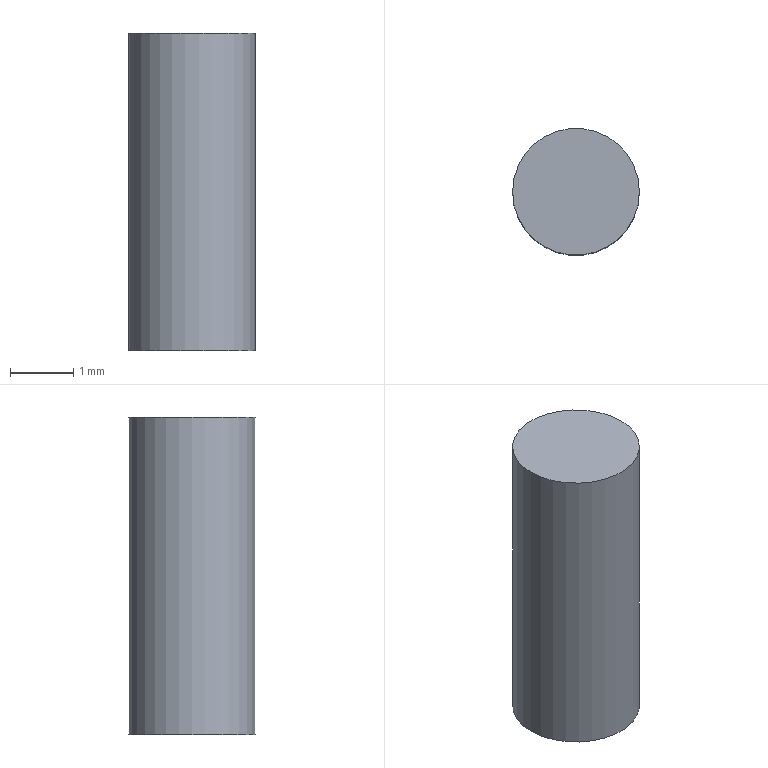Part | STEP file | SOLID | 1 solid | 3 faces | box 2 x 2 x 5 mm | volume 15.708 mm3 | plane 2 | cylinder 1 | commonest cylinder face diameters 2 x1
STEP:
#1=CARTESIAN_POINT('',(0.,0.,0.));
#2=DIRECTION('',(0.,0.,1.));
#3=DIRECTION('',(1.,0.,0.));
#4=AXIS2_PLACEMENT_3D('',#1,#2,#3);
#5=CARTESIAN_POINT('',(1.,0.,5.));
#6=VERTEX_POINT('',#5);
#7=CARTESIAN_POINT('',(0.,0.,5.));
#8=DIRECTION('',(0.,0.,1.));
#9=DIRECTION('',(1.,0.,0.));
#10=AXIS2_PLACEMENT_3D('',#7,#8,#9);
#11=CIRCLE('',#10,1.);
#12=CARTESIAN_POINT('',(0.,0.,5.));
#13=DIRECTION('',(0.,0.,-1.));
#14=DIRECTION('',(-1.,0.,0.));
#15=AXIS2_PLACEMENT_3D('',#12,#13,#14);
#16=CYLINDRICAL_SURFACE('',#15,1.);
#17=CARTESIAN_POINT('',(9.425,0.));
#18=DIRECTION('',(-1.,0.));
#19=VECTOR('',#18,1.);
#20=LINE('',#17,#19);
#21=(GEOMETRIC_REPRESENTATION_CONTEXT(2)PARAMETRIC_REPRESENTATION_CONTEXT()REPRESENTATION_CONTEXT('',''));
#22=DEFINITIONAL_REPRESENTATION('',(#20),#21);
#23=PCURVE('',#16,#22);
#24=CARTESIAN_POINT('',(0.,0.,5.));
#25=DIRECTION('',(0.,0.,1.));
#26=DIRECTION('',(1.,0.,0.));
#27=AXIS2_PLACEMENT_3D('',#24,#25,#26);
#28=PLANE('',#27);
#29=CARTESIAN_POINT('',(0.,0.));
#30=DIRECTION('',(1.,0.));
#31=AXIS2_PLACEMENT_2D('',#29,#30);
#32=CIRCLE('',#31,1.);
#33=(GEOMETRIC_REPRESENTATION_CONTEXT(2)PARAMETRIC_REPRESENTATION_CONTEXT()REPRESENTATION_CONTEXT('',''));
#34=DEFINITIONAL_REPRESENTATION('',(#32),#33);
#35=PCURVE('',#28,#34);
#36=SURFACE_CURVE('',#11,(#23,#35),.PCURVE_S1.);
#37=EDGE_CURVE('',#6,#6,#36,.T.);
#38=ORIENTED_EDGE('',*,*,#37,.F.);
#39=CARTESIAN_POINT('',(1.,0.,0.));
#40=VERTEX_POINT('',#39);
#41=CARTESIAN_POINT('',(1.,0.,5.));
#42=CARTESIAN_POINT('',(1.,0.,0.));
#43=B_SPLINE_CURVE_WITH_KNOTS('',1,(#41,#42),.UNSPECIFIED.,.F.,.F.,(2,2),(0.,5.),.PIECEWISE_BEZIER_KNOTS.);
#44=CARTESIAN_POINT('',(9.425,0.));
#45=DIRECTION('',(0.,1.));
#46=VECTOR('',#45,1.);
#47=LINE('',#44,#46);
#48=(GEOMETRIC_REPRESENTATION_CONTEXT(2)PARAMETRIC_REPRESENTATION_CONTEXT()REPRESENTATION_CONTEXT('',''));
#49=DEFINITIONAL_REPRESENTATION('',(#47),#48);
#50=PCURVE('',#16,#49);
#51=CARTESIAN_POINT('',(3.142,0.));
#52=DIRECTION('',(0.,1.));
#53=VECTOR('',#52,1.);
#54=LINE('',#51,#53);
#55=(GEOMETRIC_REPRESENTATION_CONTEXT(2)PARAMETRIC_REPRESENTATION_CONTEXT()REPRESENTATION_CONTEXT('',''));
#56=DEFINITIONAL_REPRESENTATION('',(#54),#55);
#57=PCURVE('',#16,#56);
#58=SEAM_CURVE('',#43,(#50,#57),.PCURVE_S1.);
#59=EDGE_CURVE('',#6,#40,#58,.T.);
#60=ORIENTED_EDGE('',*,*,#59,.T.);
#61=CARTESIAN_POINT('',(0.,0.,0.));
#62=DIRECTION('',(0.,0.,1.));
#63=DIRECTION('',(1.,0.,0.));
#64=AXIS2_PLACEMENT_3D('',#61,#62,#63);
#65=CIRCLE('',#64,1.);
#66=CARTESIAN_POINT('',(9.425,5.));
#67=DIRECTION('',(-1.,0.));
#68=VECTOR('',#67,1.);
#69=LINE('',#66,#68);
#70=(GEOMETRIC_REPRESENTATION_CONTEXT(2)PARAMETRIC_REPRESENTATION_CONTEXT()REPRESENTATION_CONTEXT('',''));
#71=DEFINITIONAL_REPRESENTATION('',(#69),#70);
#72=PCURVE('',#16,#71);
#73=CARTESIAN_POINT('',(0.,0.,0.));
#74=DIRECTION('',(0.,0.,1.));
#75=DIRECTION('',(1.,0.,0.));
#76=AXIS2_PLACEMENT_3D('',#73,#74,#75);
#77=PLANE('',#76);
#78=CARTESIAN_POINT('',(0.,0.));
#79=DIRECTION('',(1.,0.));
#80=AXIS2_PLACEMENT_2D('',#78,#79);
#81=CIRCLE('',#80,1.);
#82=(GEOMETRIC_REPRESENTATION_CONTEXT(2)PARAMETRIC_REPRESENTATION_CONTEXT()REPRESENTATION_CONTEXT('',''));
#83=DEFINITIONAL_REPRESENTATION('',(#81),#82);
#84=PCURVE('',#77,#83);
#85=SURFACE_CURVE('',#65,(#72,#84),.PCURVE_S1.);
#86=EDGE_CURVE('',#40,#40,#85,.T.);
#87=ORIENTED_EDGE('',*,*,#86,.T.);
#88=ORIENTED_EDGE('',*,*,#59,.F.);
#89=EDGE_LOOP('',(#38,#60,#87,#88));
#90=FACE_BOUND('',#89,.T.);
#91=ADVANCED_FACE('',(#90),#16,.T.);
#92=ORIENTED_EDGE('',*,*,#37,.T.);
#93=EDGE_LOOP('',(#92));
#94=FACE_BOUND('',#93,.T.);
#95=ADVANCED_FACE('',(#94),#28,.T.);
#96=ORIENTED_EDGE('',*,*,#86,.F.);
#97=EDGE_LOOP('',(#96));
#98=FACE_BOUND('',#97,.T.);
#99=ADVANCED_FACE('',(#98),#77,.F.);
#100=CLOSED_SHELL('',(#91,#95,#99));
#101=MANIFOLD_SOLID_BREP('',#100);
#102=(LENGTH_UNIT()NAMED_UNIT(*)SI_UNIT(.MILLI.,.METRE.));
#103=UNCERTAINTY_MEASURE_WITH_UNIT(LENGTH_MEASURE(0.00001),#102,'','');
#104=(NAMED_UNIT(*)PLANE_ANGLE_UNIT()SI_UNIT($,.RADIAN.));
#105=(NAMED_UNIT(*)SI_UNIT($,.STERADIAN.)SOLID_ANGLE_UNIT());
#106=(GEOMETRIC_REPRESENTATION_CONTEXT(3)GLOBAL_UNCERTAINTY_ASSIGNED_CONTEXT((#103))GLOBAL_UNIT_ASSIGNED_CONTEXT((#102,#104,#105))REPRESENTATION_CONTEXT('',''));
#107=ADVANCED_BREP_SHAPE_REPRESENTATION('',(#4,#101),#106);